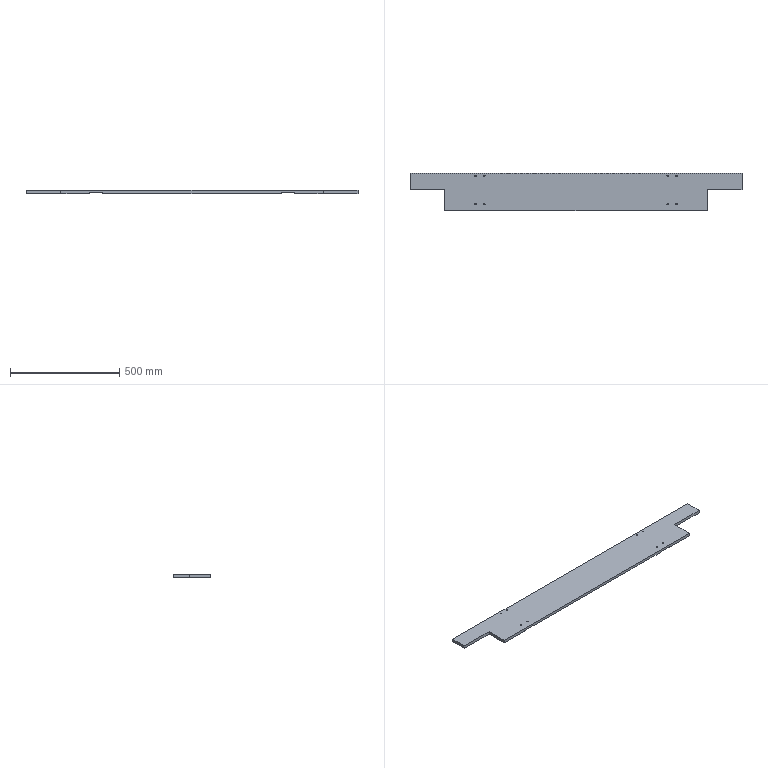Part | SolidWorks | features BaseBody 1 | 1 solid | 40 faces | box 1520 x 172 x 14 mm | volume 3159100 mm3 | cylinder 22 | plane 18 | commonest cylinder face diameters 6.8 x16 10 x6
STEP:
#1=CARTESIAN_POINT('',(-463.4,75.5,14.));
#2=VERTEX_POINT('',#1);
#3=CARTESIAN_POINT('',(-456.6,75.5,14.));
#4=VERTEX_POINT('',#3);
#5=CARTESIAN_POINT('',(-460.,75.5,14.));
#6=DIRECTION('',(0.,0.,1.));
#7=DIRECTION('',(1.,0.,0.));
#8=AXIS2_PLACEMENT_3D('',#5,#6,#7);
#9=CIRCLE('',#8,3.4);
#10=EDGE_CURVE('',#2,#4,#9,.T.);
#11=ORIENTED_EDGE('',*,*,#10,.T.);
#12=CARTESIAN_POINT('',(-456.6,75.5,3.));
#13=VERTEX_POINT('',#12);
#14=CARTESIAN_POINT('',(-456.6,75.5,3.));
#15=DIRECTION('',(0.,0.,-1.));
#16=VECTOR('',#15,1000.);
#17=LINE('',#14,#16);
#18=EDGE_CURVE('',#4,#13,#17,.T.);
#19=ORIENTED_EDGE('',*,*,#18,.T.);
#20=CARTESIAN_POINT('',(-463.4,75.5,3.));
#21=VERTEX_POINT('',#20);
#22=CARTESIAN_POINT('',(-460.,75.5,3.));
#23=DIRECTION('',(0.,0.,-1.));
#24=DIRECTION('',(-1.,0.,0.));
#25=AXIS2_PLACEMENT_3D('',#22,#23,#24);
#26=CIRCLE('',#25,3.4);
#27=EDGE_CURVE('',#13,#21,#26,.T.);
#28=ORIENTED_EDGE('',*,*,#27,.T.);
#29=CARTESIAN_POINT('',(-463.4,75.5,3.));
#30=DIRECTION('',(0.,0.,-1.));
#31=VECTOR('',#30,1000.);
#32=LINE('',#29,#31);
#33=EDGE_CURVE('',#2,#21,#32,.T.);
#34=ORIENTED_EDGE('',*,*,#33,.F.);
#35=EDGE_LOOP('',(#11,#19,#28,#34));
#36=FACE_OUTER_BOUND('',#35,.T.);
#37=CARTESIAN_POINT('',(-460.,75.5,3.));
#38=DIRECTION('',(0.,0.,-1.));
#39=DIRECTION('',(-1.,0.,0.));
#40=AXIS2_PLACEMENT_3D('',#37,#38,#39);
#41=CYLINDRICAL_SURFACE('',#40,3.4);
#42=ADVANCED_FACE('',(#36),#41,.F.);
#43=CARTESIAN_POINT('',(-423.4,75.5,14.));
#44=VERTEX_POINT('',#43);
#45=CARTESIAN_POINT('',(-416.6,75.5,14.));
#46=VERTEX_POINT('',#45);
#47=CARTESIAN_POINT('',(-420.,75.5,14.));
#48=DIRECTION('',(0.,0.,1.));
#49=DIRECTION('',(1.,0.,0.));
#50=AXIS2_PLACEMENT_3D('',#47,#48,#49);
#51=CIRCLE('',#50,3.4);
#52=EDGE_CURVE('',#44,#46,#51,.T.);
#53=ORIENTED_EDGE('',*,*,#52,.T.);
#54=CARTESIAN_POINT('',(-416.6,75.5,3.));
#55=VERTEX_POINT('',#54);
#56=CARTESIAN_POINT('',(-416.6,75.5,3.));
#57=DIRECTION('',(0.,0.,-1.));
#58=VECTOR('',#57,1000.);
#59=LINE('',#56,#58);
#60=EDGE_CURVE('',#46,#55,#59,.T.);
#61=ORIENTED_EDGE('',*,*,#60,.T.);
#62=CARTESIAN_POINT('',(-423.4,75.5,3.));
#63=VERTEX_POINT('',#62);
#64=CARTESIAN_POINT('',(-420.,75.5,3.));
#65=DIRECTION('',(0.,0.,-1.));
#66=DIRECTION('',(-1.,0.,0.));
#67=AXIS2_PLACEMENT_3D('',#64,#65,#66);
#68=CIRCLE('',#67,3.4);
#69=EDGE_CURVE('',#55,#63,#68,.T.);
#70=ORIENTED_EDGE('',*,*,#69,.T.);
#71=CARTESIAN_POINT('',(-423.4,75.5,3.));
#72=DIRECTION('',(0.,0.,-1.));
#73=VECTOR('',#72,1000.);
#74=LINE('',#71,#73);
#75=EDGE_CURVE('',#44,#63,#74,.T.);
#76=ORIENTED_EDGE('',*,*,#75,.F.);
#77=EDGE_LOOP('',(#53,#61,#70,#76));
#78=FACE_OUTER_BOUND('',#77,.T.);
#79=CARTESIAN_POINT('',(-420.,75.5,3.));
#80=DIRECTION('',(0.,0.,-1.));
#81=DIRECTION('',(-1.,0.,0.));
#82=AXIS2_PLACEMENT_3D('',#79,#80,#81);
#83=CYLINDRICAL_SURFACE('',#82,3.4);
#84=ADVANCED_FACE('',(#78),#83,.F.);
#85=CARTESIAN_POINT('',(-423.4,-54.5,14.));
#86=VERTEX_POINT('',#85);
#87=CARTESIAN_POINT('',(-416.6,-54.5,14.));
#88=VERTEX_POINT('',#87);
#89=CARTESIAN_POINT('',(-420.,-54.5,14.));
#90=DIRECTION('',(0.,0.,1.));
#91=DIRECTION('',(1.,0.,0.));
#92=AXIS2_PLACEMENT_3D('',#89,#90,#91);
#93=CIRCLE('',#92,3.4);
#94=EDGE_CURVE('',#86,#88,#93,.T.);
#95=ORIENTED_EDGE('',*,*,#94,.T.);
#96=CARTESIAN_POINT('',(-416.6,-54.5,3.));
#97=VERTEX_POINT('',#96);
#98=CARTESIAN_POINT('',(-416.6,-54.5,3.));
#99=DIRECTION('',(0.,0.,-1.));
#100=VECTOR('',#99,1000.);
#101=LINE('',#98,#100);
#102=EDGE_CURVE('',#88,#97,#101,.T.);
#103=ORIENTED_EDGE('',*,*,#102,.T.);
#104=CARTESIAN_POINT('',(-423.4,-54.5,3.));
#105=VERTEX_POINT('',#104);
#106=CARTESIAN_POINT('',(-420.,-54.5,3.));
#107=DIRECTION('',(0.,0.,-1.));
#108=DIRECTION('',(-1.,0.,0.));
#109=AXIS2_PLACEMENT_3D('',#106,#107,#108);
#110=CIRCLE('',#109,3.4);
#111=EDGE_CURVE('',#97,#105,#110,.T.);
#112=ORIENTED_EDGE('',*,*,#111,.T.);
#113=CARTESIAN_POINT('',(-423.4,-54.5,3.));
#114=DIRECTION('',(0.,0.,-1.));
#115=VECTOR('',#114,1000.);
#116=LINE('',#113,#115);
#117=EDGE_CURVE('',#86,#105,#116,.T.);
#118=ORIENTED_EDGE('',*,*,#117,.F.);
#119=EDGE_LOOP('',(#95,#103,#112,#118));
#120=FACE_OUTER_BOUND('',#119,.T.);
#121=CARTESIAN_POINT('',(-420.,-54.5,3.));
#122=DIRECTION('',(0.,0.,-1.));
#123=DIRECTION('',(-1.,0.,0.));
#124=AXIS2_PLACEMENT_3D('',#121,#122,#123);
#125=CYLINDRICAL_SURFACE('',#124,3.4);
#126=ADVANCED_FACE('',(#120),#125,.F.);
#127=CARTESIAN_POINT('',(-463.4,-54.5,14.));
#128=VERTEX_POINT('',#127);
#129=CARTESIAN_POINT('',(-456.6,-54.5,14.));
#130=VERTEX_POINT('',#129);
#131=CARTESIAN_POINT('',(-460.,-54.5,14.));
#132=DIRECTION('',(0.,0.,1.));
#133=DIRECTION('',(1.,0.,0.));
#134=AXIS2_PLACEMENT_3D('',#131,#132,#133);
#135=CIRCLE('',#134,3.4);
#136=EDGE_CURVE('',#128,#130,#135,.T.);
#137=ORIENTED_EDGE('',*,*,#136,.T.);
#138=CARTESIAN_POINT('',(-456.6,-54.5,3.));
#139=VERTEX_POINT('',#138);
#140=CARTESIAN_POINT('',(-456.6,-54.5,3.));
#141=DIRECTION('',(0.,0.,-1.));
#142=VECTOR('',#141,1000.);
#143=LINE('',#140,#142);
#144=EDGE_CURVE('',#130,#139,#143,.T.);
#145=ORIENTED_EDGE('',*,*,#144,.T.);
#146=CARTESIAN_POINT('',(-463.4,-54.5,3.));
#147=VERTEX_POINT('',#146);
#148=CARTESIAN_POINT('',(-460.,-54.5,3.));
#149=DIRECTION('',(0.,0.,-1.));
#150=DIRECTION('',(-1.,0.,0.));
#151=AXIS2_PLACEMENT_3D('',#148,#149,#150);
#152=CIRCLE('',#151,3.4);
#153=EDGE_CURVE('',#139,#147,#152,.T.);
#154=ORIENTED_EDGE('',*,*,#153,.T.);
#155=CARTESIAN_POINT('',(-463.4,-54.5,3.));
#156=DIRECTION('',(0.,0.,-1.));
#157=VECTOR('',#156,1000.);
#158=LINE('',#155,#157);
#159=EDGE_CURVE('',#128,#147,#158,.T.);
#160=ORIENTED_EDGE('',*,*,#159,.F.);
#161=EDGE_LOOP('',(#137,#145,#154,#160));
#162=FACE_OUTER_BOUND('',#161,.T.);
#163=CARTESIAN_POINT('',(-460.,-54.5,3.));
#164=DIRECTION('',(0.,0.,-1.));
#165=DIRECTION('',(-1.,0.,0.));
#166=AXIS2_PLACEMENT_3D('',#163,#164,#165);
#167=CYLINDRICAL_SURFACE('',#166,3.4);
#168=ADVANCED_FACE('',(#162),#167,.F.);
#169=CARTESIAN_POINT('',(416.6,75.5,14.));
#170=VERTEX_POINT('',#169);
#171=CARTESIAN_POINT('',(423.4,75.5,14.));
#172=VERTEX_POINT('',#171);
#173=CARTESIAN_POINT('',(420.,75.5,14.));
#174=DIRECTION('',(0.,0.,1.));
#175=DIRECTION('',(1.,0.,0.));
#176=AXIS2_PLACEMENT_3D('',#173,#174,#175);
#177=CIRCLE('',#176,3.4);
#178=EDGE_CURVE('',#170,#172,#177,.T.);
#179=ORIENTED_EDGE('',*,*,#178,.T.);
#180=CARTESIAN_POINT('',(423.4,75.5,3.));
#181=VERTEX_POINT('',#180);
#182=CARTESIAN_POINT('',(423.4,75.5,3.));
#183=DIRECTION('',(0.,0.,-1.));
#184=VECTOR('',#183,1000.);
#185=LINE('',#182,#184);
#186=EDGE_CURVE('',#172,#181,#185,.T.);
#187=ORIENTED_EDGE('',*,*,#186,.T.);
#188=CARTESIAN_POINT('',(416.6,75.5,3.));
#189=VERTEX_POINT('',#188);
#190=CARTESIAN_POINT('',(420.,75.5,3.));
#191=DIRECTION('',(0.,0.,-1.));
#192=DIRECTION('',(-1.,0.,0.));
#193=AXIS2_PLACEMENT_3D('',#190,#191,#192);
#194=CIRCLE('',#193,3.4);
#195=EDGE_CURVE('',#181,#189,#194,.T.);
#196=ORIENTED_EDGE('',*,*,#195,.T.);
#197=CARTESIAN_POINT('',(416.6,75.5,3.));
#198=DIRECTION('',(0.,0.,-1.));
#199=VECTOR('',#198,1000.);
#200=LINE('',#197,#199);
#201=EDGE_CURVE('',#170,#189,#200,.T.);
#202=ORIENTED_EDGE('',*,*,#201,.F.);
#203=EDGE_LOOP('',(#179,#187,#196,#202));
#204=FACE_OUTER_BOUND('',#203,.T.);
#205=CARTESIAN_POINT('',(420.,75.5,3.));
#206=DIRECTION('',(0.,0.,-1.));
#207=DIRECTION('',(-1.,0.,0.));
#208=AXIS2_PLACEMENT_3D('',#205,#206,#207);
#209=CYLINDRICAL_SURFACE('',#208,3.4);
#210=ADVANCED_FACE('',(#204),#209,.F.);
#211=CARTESIAN_POINT('',(456.6,75.5,14.));
#212=VERTEX_POINT('',#211);
#213=CARTESIAN_POINT('',(463.4,75.5,14.));
#214=VERTEX_POINT('',#213);
#215=CARTESIAN_POINT('',(460.,75.5,14.));
#216=DIRECTION('',(0.,0.,1.));
#217=DIRECTION('',(1.,0.,0.));
#218=AXIS2_PLACEMENT_3D('',#215,#216,#217);
#219=CIRCLE('',#218,3.4);
#220=EDGE_CURVE('',#212,#214,#219,.T.);
#221=ORIENTED_EDGE('',*,*,#220,.T.);
#222=CARTESIAN_POINT('',(463.4,75.5,3.));
#223=VERTEX_POINT('',#222);
#224=CARTESIAN_POINT('',(463.4,75.5,3.));
#225=DIRECTION('',(0.,0.,-1.));
#226=VECTOR('',#225,1000.);
#227=LINE('',#224,#226);
#228=EDGE_CURVE('',#214,#223,#227,.T.);
#229=ORIENTED_EDGE('',*,*,#228,.T.);
#230=CARTESIAN_POINT('',(456.6,75.5,3.));
#231=VERTEX_POINT('',#230);
#232=CARTESIAN_POINT('',(460.,75.5,3.));
#233=DIRECTION('',(0.,0.,-1.));
#234=DIRECTION('',(-1.,0.,0.));
#235=AXIS2_PLACEMENT_3D('',#232,#233,#234);
#236=CIRCLE('',#235,3.4);
#237=EDGE_CURVE('',#223,#231,#236,.T.);
#238=ORIENTED_EDGE('',*,*,#237,.T.);
#239=CARTESIAN_POINT('',(456.6,75.5,3.));
#240=DIRECTION('',(0.,0.,-1.));
#241=VECTOR('',#240,1000.);
#242=LINE('',#239,#241);
#243=EDGE_CURVE('',#212,#231,#242,.T.);
#244=ORIENTED_EDGE('',*,*,#243,.F.);
#245=EDGE_LOOP('',(#221,#229,#238,#244));
#246=FACE_OUTER_BOUND('',#245,.T.);
#247=CARTESIAN_POINT('',(460.,75.5,3.));
#248=DIRECTION('',(0.,0.,-1.));
#249=DIRECTION('',(-1.,0.,0.));
#250=AXIS2_PLACEMENT_3D('',#247,#248,#249);
#251=CYLINDRICAL_SURFACE('',#250,3.4);
#252=ADVANCED_FACE('',(#246),#251,.F.);
#253=CARTESIAN_POINT('',(456.6,-54.5,14.));
#254=VERTEX_POINT('',#253);
#255=CARTESIAN_POINT('',(463.4,-54.5,14.));
#256=VERTEX_POINT('',#255);
#257=CARTESIAN_POINT('',(460.,-54.5,14.));
#258=DIRECTION('',(0.,0.,1.));
#259=DIRECTION('',(1.,0.,0.));
#260=AXIS2_PLACEMENT_3D('',#257,#258,#259);
#261=CIRCLE('',#260,3.4);
#262=EDGE_CURVE('',#254,#256,#261,.T.);
#263=ORIENTED_EDGE('',*,*,#262,.T.);
#264=CARTESIAN_POINT('',(463.4,-54.5,3.));
#265=VERTEX_POINT('',#264);
#266=CARTESIAN_POINT('',(463.4,-54.5,3.));
#267=DIRECTION('',(0.,0.,-1.));
#268=VECTOR('',#267,1000.);
#269=LINE('',#266,#268);
#270=EDGE_CURVE('',#256,#265,#269,.T.);
#271=ORIENTED_EDGE('',*,*,#270,.T.);
#272=CARTESIAN_POINT('',(456.6,-54.5,3.));
#273=VERTEX_POINT('',#272);
#274=CARTESIAN_POINT('',(460.,-54.5,3.));
#275=DIRECTION('',(0.,0.,-1.));
#276=DIRECTION('',(-1.,0.,0.));
#277=AXIS2_PLACEMENT_3D('',#274,#275,#276);
#278=CIRCLE('',#277,3.4);
#279=EDGE_CURVE('',#265,#273,#278,.T.);
#280=ORIENTED_EDGE('',*,*,#279,.T.);
#281=CARTESIAN_POINT('',(456.6,-54.5,3.));
#282=DIRECTION('',(0.,0.,-1.));
#283=VECTOR('',#282,1000.);
#284=LINE('',#281,#283);
#285=EDGE_CURVE('',#254,#273,#284,.T.);
#286=ORIENTED_EDGE('',*,*,#285,.F.);
#287=EDGE_LOOP('',(#263,#271,#280,#286));
#288=FACE_OUTER_BOUND('',#287,.T.);
#289=CARTESIAN_POINT('',(460.,-54.5,3.));
#290=DIRECTION('',(0.,0.,-1.));
#291=DIRECTION('',(-1.,0.,0.));
#292=AXIS2_PLACEMENT_3D('',#289,#290,#291);
#293=CYLINDRICAL_SURFACE('',#292,3.4);
#294=ADVANCED_FACE('',(#288),#293,.F.);
#295=CARTESIAN_POINT('',(416.6,-54.5,14.));
#296=VERTEX_POINT('',#295);
#297=CARTESIAN_POINT('',(423.4,-54.5,14.));
#298=VERTEX_POINT('',#297);
#299=CARTESIAN_POINT('',(420.,-54.5,14.));
#300=DIRECTION('',(0.,0.,1.));
#301=DIRECTION('',(1.,0.,0.));
#302=AXIS2_PLACEMENT_3D('',#299,#300,#301);
#303=CIRCLE('',#302,3.4);
#304=EDGE_CURVE('',#296,#298,#303,.T.);
#305=ORIENTED_EDGE('',*,*,#304,.T.);
#306=CARTESIAN_POINT('',(423.4,-54.5,3.));
#307=VERTEX_POINT('',#306);
#308=CARTESIAN_POINT('',(423.4,-54.5,3.));
#309=DIRECTION('',(0.,0.,-1.));
#310=VECTOR('',#309,1000.);
#311=LINE('',#308,#310);
#312=EDGE_CURVE('',#298,#307,#311,.T.);
#313=ORIENTED_EDGE('',*,*,#312,.T.);
#314=CARTESIAN_POINT('',(416.6,-54.5,3.));
#315=VERTEX_POINT('',#314);
#316=CARTESIAN_POINT('',(420.,-54.5,3.));
#317=DIRECTION('',(0.,0.,-1.));
#318=DIRECTION('',(-1.,0.,0.));
#319=AXIS2_PLACEMENT_3D('',#316,#317,#318);
#320=CIRCLE('',#319,3.4);
#321=EDGE_CURVE('',#307,#315,#320,.T.);
#322=ORIENTED_EDGE('',*,*,#321,.T.);
#323=CARTESIAN_POINT('',(416.6,-54.5,3.));
#324=DIRECTION('',(0.,0.,-1.));
#325=VECTOR('',#324,1000.);
#326=LINE('',#323,#325);
#327=EDGE_CURVE('',#296,#315,#326,.T.);
#328=ORIENTED_EDGE('',*,*,#327,.F.);
#329=EDGE_LOOP('',(#305,#313,#322,#328));
#330=FACE_OUTER_BOUND('',#329,.T.);
#331=CARTESIAN_POINT('',(420.,-54.5,3.));
#332=DIRECTION('',(0.,0.,-1.));
#333=DIRECTION('',(-1.,0.,0.));
#334=AXIS2_PLACEMENT_3D('',#331,#332,#333);
#335=CYLINDRICAL_SURFACE('',#334,3.4);
#336=ADVANCED_FACE('',(#330),#335,.F.);
#337=CARTESIAN_POINT('',(-475.5,85.5,3.));
#338=VERTEX_POINT('',#337);
#339=CARTESIAN_POINT('',(-475.083,87.5,3.));
#340=VERTEX_POINT('',#339);
#341=CARTESIAN_POINT('',(-470.5,85.5,3.));
#342=DIRECTION('',(0.,0.,-1.));
#343=DIRECTION('',(1.,0.,0.));
#344=AXIS2_PLACEMENT_3D('',#341,#342,#343);
#345=CIRCLE('',#344,5.);
#346=EDGE_CURVE('',#338,#340,#345,.T.);
#347=ORIENTED_EDGE('',*,*,#346,.F.);
#348=CARTESIAN_POINT('',(-475.5,85.5,0.));
#349=VERTEX_POINT('',#348);
#350=CARTESIAN_POINT('',(-475.5,85.5,3.));
#351=DIRECTION('',(0.,0.,-1.));
#352=VECTOR('',#351,1000.);
#353=LINE('',#350,#352);
#354=EDGE_CURVE('',#338,#349,#353,.T.);
#355=ORIENTED_EDGE('',*,*,#354,.T.);
#356=CARTESIAN_POINT('',(-475.083,87.5,0.));
#357=VERTEX_POINT('',#356);
#358=CARTESIAN_POINT('',(-470.5,85.5,0.));
#359=DIRECTION('',(0.,0.,1.));
#360=DIRECTION('',(1.,0.,0.));
#361=AXIS2_PLACEMENT_3D('',#358,#359,#360);
#362=CIRCLE('',#361,5.);
#363=EDGE_CURVE('',#357,#349,#362,.T.);
#364=ORIENTED_EDGE('',*,*,#363,.F.);
#365=CARTESIAN_POINT('',(-475.083,87.5,3.));
#366=DIRECTION('',(0.,0.,-1.));
#367=VECTOR('',#366,1000.);
#368=LINE('',#365,#367);
#369=EDGE_CURVE('',#340,#357,#368,.T.);
#370=ORIENTED_EDGE('',*,*,#369,.F.);
#371=EDGE_LOOP('',(#347,#355,#364,#370));
#372=FACE_OUTER_BOUND('',#371,.T.);
#373=CARTESIAN_POINT('',(-470.5,85.5,3.));
#374=DIRECTION('',(0.,0.,-1.));
#375=DIRECTION('',(-1.,0.,0.));
#376=AXIS2_PLACEMENT_3D('',#373,#374,#375);
#377=CYLINDRICAL_SURFACE('',#376,5.);
#378=ADVANCED_FACE('',(#372),#377,.F.);
#379=CARTESIAN_POINT('',(404.5,85.5,3.));
#380=VERTEX_POINT('',#379);
#381=CARTESIAN_POINT('',(404.917,87.5,3.));
#382=VERTEX_POINT('',#381);
#383=CARTESIAN_POINT('',(409.5,85.5,3.));
#384=DIRECTION('',(0.,0.,-1.));
#385=DIRECTION('',(-1.,0.,0.));
#386=AXIS2_PLACEMENT_3D('',#383,#384,#385);
#387=CIRCLE('',#386,5.);
#388=EDGE_CURVE('',#380,#382,#387,.T.);
#389=ORIENTED_EDGE('',*,*,#388,.F.);
#390=CARTESIAN_POINT('',(404.5,85.5,0.));
#391=VERTEX_POINT('',#390);
#392=CARTESIAN_POINT('',(404.5,85.5,3.));
#393=DIRECTION('',(0.,0.,-1.));
#394=VECTOR('',#393,1000.);
#395=LINE('',#392,#394);
#396=EDGE_CURVE('',#380,#391,#395,.T.);
#397=ORIENTED_EDGE('',*,*,#396,.T.);
#398=CARTESIAN_POINT('',(404.917,87.5,0.));
#399=VERTEX_POINT('',#398);
#400=CARTESIAN_POINT('',(409.5,85.5,0.));
#401=DIRECTION('',(0.,0.,1.));
#402=DIRECTION('',(1.,0.,0.));
#403=AXIS2_PLACEMENT_3D('',#400,#401,#402);
#404=CIRCLE('',#403,5.);
#405=EDGE_CURVE('',#399,#391,#404,.T.);
#406=ORIENTED_EDGE('',*,*,#405,.F.);
#407=CARTESIAN_POINT('',(404.917,87.5,3.));
#408=DIRECTION('',(0.,0.,-1.));
#409=VECTOR('',#408,1000.);
#410=LINE('',#407,#409);
#411=EDGE_CURVE('',#382,#399,#410,.T.);
#412=ORIENTED_EDGE('',*,*,#411,.F.);
#413=EDGE_LOOP('',(#389,#397,#406,#412));
#414=FACE_OUTER_BOUND('',#413,.T.);
#415=CARTESIAN_POINT('',(409.5,85.5,3.));
#416=DIRECTION('',(0.,0.,-1.));
#417=DIRECTION('',(-1.,0.,0.));
#418=AXIS2_PLACEMENT_3D('',#415,#416,#417);
#419=CYLINDRICAL_SURFACE('',#418,5.);
#420=ADVANCED_FACE('',(#414),#419,.F.);
#421=CARTESIAN_POINT('',(-409.5,80.5,0.));
#422=VERTEX_POINT('',#421);
#423=CARTESIAN_POINT('',(-409.5,-84.5,0.));
#424=VERTEX_POINT('',#423);
#425=CARTESIAN_POINT('',(-409.5,0.,0.));
#426=DIRECTION('',(0.,-1.,0.));
#427=VECTOR('',#426,1000.);
#428=LINE('',#425,#427);
#429=EDGE_CURVE('',#422,#424,#428,.T.);
#430=ORIENTED_EDGE('',*,*,#429,.F.);
#431=CARTESIAN_POINT('',(-404.917,87.5,0.));
#432=VERTEX_POINT('',#431);
#433=CARTESIAN_POINT('',(-409.5,85.5,0.));
#434=DIRECTION('',(0.,0.,1.));
#435=DIRECTION('',(1.,0.,0.));
#436=AXIS2_PLACEMENT_3D('',#433,#434,#435);
#437=CIRCLE('',#436,5.);
#438=EDGE_CURVE('',#422,#432,#437,.T.);
#439=ORIENTED_EDGE('',*,*,#438,.T.);
#440=CARTESIAN_POINT('',(-760.,87.5,0.));
#441=DIRECTION('',(-1.,0.,0.));
#442=VECTOR('',#441,1000.);
#443=LINE('',#440,#442);
#444=EDGE_CURVE('',#399,#432,#443,.T.);
#445=ORIENTED_EDGE('',*,*,#444,.F.);
#446=ORIENTED_EDGE('',*,*,#405,.T.);
#447=CARTESIAN_POINT('',(409.5,80.5,0.));
#448=VERTEX_POINT('',#447);
#449=CARTESIAN_POINT('',(409.5,85.5,0.));
#450=DIRECTION('',(0.,0.,1.));
#451=DIRECTION('',(1.,0.,0.));
#452=AXIS2_PLACEMENT_3D('',#449,#450,#451);
#453=CIRCLE('',#452,5.);
#454=EDGE_CURVE('',#391,#448,#453,.T.);
#455=ORIENTED_EDGE('',*,*,#454,.T.);
#456=CARTESIAN_POINT('',(409.5,-84.5,0.));
#457=VERTEX_POINT('',#456);
#458=CARTESIAN_POINT('',(409.5,0.,0.));
#459=DIRECTION('',(0.,1.,0.));
#460=VECTOR('',#459,1000.);
#461=LINE('',#458,#460);
#462=EDGE_CURVE('',#457,#448,#461,.T.);
#463=ORIENTED_EDGE('',*,*,#462,.F.);
#464=CARTESIAN_POINT('',(-600.,-84.5,0.));
#465=DIRECTION('',(1.,0.,0.));
#466=VECTOR('',#465,1000.);
#467=LINE('',#464,#466);
#468=EDGE_CURVE('',#424,#457,#467,.T.);
#469=ORIENTED_EDGE('',*,*,#468,.F.);
#470=EDGE_LOOP('',(#430,#439,#445,#446,#455,#463,#469));
#471=FACE_OUTER_BOUND('',#470,.T.);
#472=CARTESIAN_POINT('',(0.,0.,0.));
#473=DIRECTION('',(0.,0.,1.));
#474=DIRECTION('',(1.,0.,0.));
#475=AXIS2_PLACEMENT_3D('',#472,#473,#474);
#476=PLANE('',#475);
#477=ADVANCED_FACE('',(#471),#476,.F.);
#478=CARTESIAN_POINT('',(470.5,80.5,0.));
#479=VERTEX_POINT('',#478);
#480=CARTESIAN_POINT('',(470.5,-84.5,0.));
#481=VERTEX_POINT('',#480);
#482=CARTESIAN_POINT('',(470.5,0.,0.));
#483=DIRECTION('',(0.,-1.,0.));
#484=VECTOR('',#483,1000.);
#485=LINE('',#482,#484);
#486=EDGE_CURVE('',#479,#481,#485,.T.);
#487=ORIENTED_EDGE('',*,*,#486,.F.);
#488=CARTESIAN_POINT('',(475.083,87.5,0.));
#489=VERTEX_POINT('',#488);
#490=CARTESIAN_POINT('',(470.5,85.5,0.));
#491=DIRECTION('',(0.,0.,1.));
#492=DIRECTION('',(1.,0.,0.));
#493=AXIS2_PLACEMENT_3D('',#490,#491,#492);
#494=CIRCLE('',#493,5.);
#495=EDGE_CURVE('',#479,#489,#494,.T.);
#496=ORIENTED_EDGE('',*,*,#495,.T.);
#497=CARTESIAN_POINT('',(760.,87.5,0.));
#498=VERTEX_POINT('',#497);
#499=CARTESIAN_POINT('',(-760.,87.5,0.));
#500=DIRECTION('',(-1.,0.,0.));
#501=VECTOR('',#500,1000.);
#502=LINE('',#499,#501);
#503=EDGE_CURVE('',#498,#489,#502,.T.);
#504=ORIENTED_EDGE('',*,*,#503,.F.);
#505=CARTESIAN_POINT('',(760.,12.5,0.));
#506=VERTEX_POINT('',#505);
#507=CARTESIAN_POINT('',(760.,87.5,0.));
#508=DIRECTION('',(0.,1.,0.));
#509=VECTOR('',#508,1000.);
#510=LINE('',#507,#509);
#511=EDGE_CURVE('',#506,#498,#510,.T.);
#512=ORIENTED_EDGE('',*,*,#511,.F.);
#513=CARTESIAN_POINT('',(600.,12.5,0.));
#514=VERTEX_POINT('',#513);
#515=CARTESIAN_POINT('',(760.,12.5,0.));
#516=DIRECTION('',(-1.,0.,0.));
#517=VECTOR('',#516,1000.);
#518=LINE('',#515,#517);
#519=EDGE_CURVE('',#506,#514,#518,.T.);
#520=ORIENTED_EDGE('',*,*,#519,.T.);
#521=CARTESIAN_POINT('',(600.,-84.5,0.));
#522=VERTEX_POINT('',#521);
#523=CARTESIAN_POINT('',(600.,12.5,0.));
#524=DIRECTION('',(0.,-1.,0.));
#525=VECTOR('',#524,1000.);
#526=LINE('',#523,#525);
#527=EDGE_CURVE('',#514,#522,#526,.T.);
#528=ORIENTED_EDGE('',*,*,#527,.T.);
#529=CARTESIAN_POINT('',(-600.,-84.5,0.));
#530=DIRECTION('',(1.,0.,0.));
#531=VECTOR('',#530,1000.);
#532=LINE('',#529,#531);
#533=EDGE_CURVE('',#481,#522,#532,.T.);
#534=ORIENTED_EDGE('',*,*,#533,.F.);
#535=EDGE_LOOP('',(#487,#496,#504,#512,#520,#528,#534));
#536=FACE_OUTER_BOUND('',#535,.T.);
#537=CARTESIAN_POINT('',(0.,0.,0.));
#538=DIRECTION('',(0.,0.,1.));
#539=DIRECTION('',(1.,0.,0.));
#540=AXIS2_PLACEMENT_3D('',#537,#538,#539);
#541=PLANE('',#540);
#542=ADVANCED_FACE('',(#536),#541,.F.);
#543=ORIENTED_EDGE('',*,*,#444,.T.);
#544=CARTESIAN_POINT('',(-404.917,87.5,3.));
#545=VERTEX_POINT('',#544);
#546=CARTESIAN_POINT('',(-404.917,87.5,3.));
#547=DIRECTION('',(0.,0.,1.));
#548=VECTOR('',#547,1000.);
#549=LINE('',#546,#548);
#550=EDGE_CURVE('',#432,#545,#549,.T.);
#551=ORIENTED_EDGE('',*,*,#550,.T.);
#552=CARTESIAN_POINT('',(-760.,87.5,3.));
#553=DIRECTION('',(-1.,0.,0.));
#554=VECTOR('',#553,1000.);
#555=LINE('',#552,#554);
#556=EDGE_CURVE('',#545,#340,#555,.T.);
#557=ORIENTED_EDGE('',*,*,#556,.T.);
#558=ORIENTED_EDGE('',*,*,#369,.T.);
#559=CARTESIAN_POINT('',(-760.,87.5,0.));
#560=VERTEX_POINT('',#559);
#561=CARTESIAN_POINT('',(-760.,87.5,0.));
#562=DIRECTION('',(-1.,0.,0.));
#563=VECTOR('',#562,1000.);
#564=LINE('',#561,#563);
#565=EDGE_CURVE('',#357,#560,#564,.T.);
#566=ORIENTED_EDGE('',*,*,#565,.T.);
#567=CARTESIAN_POINT('',(-760.,87.5,14.));
#568=VERTEX_POINT('',#567);
#569=CARTESIAN_POINT('',(-760.,87.5,14.));
#570=DIRECTION('',(0.,0.,-1.));
#571=VECTOR('',#570,1000.);
#572=LINE('',#569,#571);
#573=EDGE_CURVE('',#568,#560,#572,.T.);
#574=ORIENTED_EDGE('',*,*,#573,.F.);
#575=CARTESIAN_POINT('',(760.,87.5,14.));
#576=VERTEX_POINT('',#575);
#577=CARTESIAN_POINT('',(-760.,87.5,14.));
#578=DIRECTION('',(-1.,0.,0.));
#579=VECTOR('',#578,1000.);
#580=LINE('',#577,#579);
#581=EDGE_CURVE('',#576,#568,#580,.T.);
#582=ORIENTED_EDGE('',*,*,#581,.F.);
#583=CARTESIAN_POINT('',(760.,87.5,14.));
#584=DIRECTION('',(0.,0.,-1.));
#585=VECTOR('',#584,1000.);
#586=LINE('',#583,#585);
#587=EDGE_CURVE('',#576,#498,#586,.T.);
#588=ORIENTED_EDGE('',*,*,#587,.T.);
#589=ORIENTED_EDGE('',*,*,#503,.T.);
#590=CARTESIAN_POINT('',(475.083,87.5,3.));
#591=VERTEX_POINT('',#590);
#592=CARTESIAN_POINT('',(475.083,87.5,3.));
#593=DIRECTION('',(0.,0.,1.));
#594=VECTOR('',#593,1000.);
#595=LINE('',#592,#594);
#596=EDGE_CURVE('',#489,#591,#595,.T.);
#597=ORIENTED_EDGE('',*,*,#596,.T.);
#598=CARTESIAN_POINT('',(-760.,87.5,3.));
#599=DIRECTION('',(-1.,0.,0.));
#600=VECTOR('',#599,1000.);
#601=LINE('',#598,#600);
#602=EDGE_CURVE('',#591,#382,#601,.T.);
#603=ORIENTED_EDGE('',*,*,#602,.T.);
#604=ORIENTED_EDGE('',*,*,#411,.T.);
#605=EDGE_LOOP('',(#543,#551,#557,#558,#566,#574,#582,#588,#589,#597,#603,#604));
#606=FACE_OUTER_BOUND('',#605,.T.);
#607=CARTESIAN_POINT('',(-760.,87.5,14.));
#608=DIRECTION('',(0.,-1.,0.));
#609=DIRECTION('',(0.,0.,-1.));
#610=AXIS2_PLACEMENT_3D('',#607,#608,#609);
#611=PLANE('',#610);
#612=ADVANCED_FACE('',(#606),#611,.F.);
#613=ORIENTED_EDGE('',*,*,#468,.T.);
#614=CARTESIAN_POINT('',(409.5,-84.5,3.));
#615=VERTEX_POINT('',#614);
#616=CARTESIAN_POINT('',(409.5,-84.5,3.));
#617=DIRECTION('',(0.,0.,-1.));
#618=VECTOR('',#617,1000.);
#619=LINE('',#616,#618);
#620=EDGE_CURVE('',#615,#457,#619,.T.);
#621=ORIENTED_EDGE('',*,*,#620,.F.);
#622=CARTESIAN_POINT('',(470.5,-84.5,3.));
#623=VERTEX_POINT('',#622);
#624=CARTESIAN_POINT('',(470.5,-84.5,3.));
#625=DIRECTION('',(1.,0.,0.));
#626=VECTOR('',#625,1000.);
#627=LINE('',#624,#626);
#628=EDGE_CURVE('',#615,#623,#627,.T.);
#629=ORIENTED_EDGE('',*,*,#628,.T.);
#630=CARTESIAN_POINT('',(470.5,-84.5,3.));
#631=DIRECTION('',(0.,0.,-1.));
#632=VECTOR('',#631,1000.);
#633=LINE('',#630,#632);
#634=EDGE_CURVE('',#623,#481,#633,.T.);
#635=ORIENTED_EDGE('',*,*,#634,.T.);
#636=ORIENTED_EDGE('',*,*,#533,.T.);
#637=CARTESIAN_POINT('',(600.,-84.5,14.));
#638=VERTEX_POINT('',#637);
#639=CARTESIAN_POINT('',(600.,-84.5,140.));
#640=DIRECTION('',(0.,0.,1.));
#641=VECTOR('',#640,1000.);
#642=LINE('',#639,#641);
#643=EDGE_CURVE('',#522,#638,#642,.T.);
#644=ORIENTED_EDGE('',*,*,#643,.T.);
#645=CARTESIAN_POINT('',(-600.,-84.5,14.));
#646=VERTEX_POINT('',#645);
#647=CARTESIAN_POINT('',(0.,-84.5,14.));
#648=DIRECTION('',(1.,0.,0.));
#649=VECTOR('',#648,1000.);
#650=LINE('',#647,#649);
#651=EDGE_CURVE('',#646,#638,#650,.T.);
#652=ORIENTED_EDGE('',*,*,#651,.F.);
#653=CARTESIAN_POINT('',(-600.,-84.5,0.));
#654=VERTEX_POINT('',#653);
#655=CARTESIAN_POINT('',(-600.,-84.5,0.));
#656=DIRECTION('',(0.,0.,-1.));
#657=VECTOR('',#656,1000.);
#658=LINE('',#655,#657);
#659=EDGE_CURVE('',#646,#654,#658,.T.);
#660=ORIENTED_EDGE('',*,*,#659,.T.);
#661=CARTESIAN_POINT('',(-470.5,-84.5,0.));
#662=VERTEX_POINT('',#661);
#663=CARTESIAN_POINT('',(-600.,-84.5,0.));
#664=DIRECTION('',(1.,0.,0.));
#665=VECTOR('',#664,1000.);
#666=LINE('',#663,#665);
#667=EDGE_CURVE('',#654,#662,#666,.T.);
#668=ORIENTED_EDGE('',*,*,#667,.T.);
#669=CARTESIAN_POINT('',(-470.5,-84.5,3.));
#670=VERTEX_POINT('',#669);
#671=CARTESIAN_POINT('',(-470.5,-84.5,3.));
#672=DIRECTION('',(0.,0.,-1.));
#673=VECTOR('',#672,1000.);
#674=LINE('',#671,#673);
#675=EDGE_CURVE('',#670,#662,#674,.T.);
#676=ORIENTED_EDGE('',*,*,#675,.F.);
#677=CARTESIAN_POINT('',(-409.5,-84.5,3.));
#678=VERTEX_POINT('',#677);
#679=CARTESIAN_POINT('',(-470.5,-84.5,3.));
#680=DIRECTION('',(1.,0.,0.));
#681=VECTOR('',#680,1000.);
#682=LINE('',#679,#681);
#683=EDGE_CURVE('',#670,#678,#682,.T.);
#684=ORIENTED_EDGE('',*,*,#683,.T.);
#685=CARTESIAN_POINT('',(-409.5,-84.5,3.));
#686=DIRECTION('',(0.,0.,-1.));
#687=VECTOR('',#686,1000.);
#688=LINE('',#685,#687);
#689=EDGE_CURVE('',#678,#424,#688,.T.);
#690=ORIENTED_EDGE('',*,*,#689,.T.);
#691=EDGE_LOOP('',(#613,#621,#629,#635,#636,#644,#652,#660,#668,#676,#684,#690));
#692=FACE_OUTER_BOUND('',#691,.T.);
#693=CARTESIAN_POINT('',(0.,-84.5,70.));
#694=DIRECTION('',(0.,-1.,0.));
#695=DIRECTION('',(0.,0.,-1.));
#696=AXIS2_PLACEMENT_3D('',#693,#694,#695);
#697=PLANE('',#696);
#698=ADVANCED_FACE('',(#692),#697,.T.);
#699=ORIENTED_EDGE('',*,*,#565,.F.);
#700=ORIENTED_EDGE('',*,*,#363,.T.);
#701=CARTESIAN_POINT('',(-470.5,80.5,0.));
#702=VERTEX_POINT('',#701);
#703=CARTESIAN_POINT('',(-470.5,85.5,0.));
#704=DIRECTION('',(0.,0.,1.));
#705=DIRECTION('',(1.,0.,0.));
#706=AXIS2_PLACEMENT_3D('',#703,#704,#705);
#707=CIRCLE('',#706,5.);
#708=EDGE_CURVE('',#349,#702,#707,.T.);
#709=ORIENTED_EDGE('',*,*,#708,.T.);
#710=CARTESIAN_POINT('',(-470.5,0.,0.));
#711=DIRECTION('',(0.,1.,0.));
#712=VECTOR('',#711,1000.);
#713=LINE('',#710,#712);
#714=EDGE_CURVE('',#662,#702,#713,.T.);
#715=ORIENTED_EDGE('',*,*,#714,.F.);
#716=ORIENTED_EDGE('',*,*,#667,.F.);
#717=CARTESIAN_POINT('',(-600.,12.5,0.));
#718=VERTEX_POINT('',#717);
#719=CARTESIAN_POINT('',(-600.,12.5,0.));
#720=DIRECTION('',(0.,1.,0.));
#721=VECTOR('',#720,1000.);
#722=LINE('',#719,#721);
#723=EDGE_CURVE('',#654,#718,#722,.T.);
#724=ORIENTED_EDGE('',*,*,#723,.T.);
#725=CARTESIAN_POINT('',(-760.,12.5,0.));
#726=VERTEX_POINT('',#725);
#727=CARTESIAN_POINT('',(-760.,12.5,0.));
#728=DIRECTION('',(-1.,0.,0.));
#729=VECTOR('',#728,1000.);
#730=LINE('',#727,#729);
#731=EDGE_CURVE('',#718,#726,#730,.T.);
#732=ORIENTED_EDGE('',*,*,#731,.T.);
#733=CARTESIAN_POINT('',(-760.,87.5,0.));
#734=DIRECTION('',(0.,-1.,0.));
#735=VECTOR('',#734,1000.);
#736=LINE('',#733,#735);
#737=EDGE_CURVE('',#560,#726,#736,.T.);
#738=ORIENTED_EDGE('',*,*,#737,.F.);
#739=EDGE_LOOP('',(#699,#700,#709,#715,#716,#724,#732,#738));
#740=FACE_OUTER_BOUND('',#739,.T.);
#741=CARTESIAN_POINT('',(0.,0.,0.));
#742=DIRECTION('',(0.,0.,1.));
#743=DIRECTION('',(1.,0.,0.));
#744=AXIS2_PLACEMENT_3D('',#741,#742,#743);
#745=PLANE('',#744);
#746=ADVANCED_FACE('',(#740),#745,.F.);
#747=ORIENTED_EDGE('',*,*,#10,.F.);
#748=CARTESIAN_POINT('',(-460.,75.5,14.));
#749=DIRECTION('',(0.,0.,1.));
#750=DIRECTION('',(1.,0.,0.));
#751=AXIS2_PLACEMENT_3D('',#748,#749,#750);
#752=CIRCLE('',#751,3.4);
#753=EDGE_CURVE('',#4,#2,#752,.T.);
#754=ORIENTED_EDGE('',*,*,#753,.F.);
#755=EDGE_LOOP('',(#747,#754));
#756=FACE_BOUND('',#755,.T.);
#757=ORIENTED_EDGE('',*,*,#52,.F.);
#758=CARTESIAN_POINT('',(-420.,75.5,14.));
#759=DIRECTION('',(0.,0.,1.));
#760=DIRECTION('',(1.,0.,0.));
#761=AXIS2_PLACEMENT_3D('',#758,#759,#760);
#762=CIRCLE('',#761,3.4);
#763=EDGE_CURVE('',#46,#44,#762,.T.);
#764=ORIENTED_EDGE('',*,*,#763,.F.);
#765=EDGE_LOOP('',(#757,#764));
#766=FACE_BOUND('',#765,.T.);
#767=ORIENTED_EDGE('',*,*,#94,.F.);
#768=CARTESIAN_POINT('',(-420.,-54.5,14.));
#769=DIRECTION('',(0.,0.,1.));
#770=DIRECTION('',(1.,0.,0.));
#771=AXIS2_PLACEMENT_3D('',#768,#769,#770);
#772=CIRCLE('',#771,3.4);
#773=EDGE_CURVE('',#88,#86,#772,.T.);
#774=ORIENTED_EDGE('',*,*,#773,.F.);
#775=EDGE_LOOP('',(#767,#774));
#776=FACE_BOUND('',#775,.T.);
#777=ORIENTED_EDGE('',*,*,#136,.F.);
#778=CARTESIAN_POINT('',(-460.,-54.5,14.));
#779=DIRECTION('',(0.,0.,1.));
#780=DIRECTION('',(1.,0.,0.));
#781=AXIS2_PLACEMENT_3D('',#778,#779,#780);
#782=CIRCLE('',#781,3.4);
#783=EDGE_CURVE('',#130,#128,#782,.T.);
#784=ORIENTED_EDGE('',*,*,#783,.F.);
#785=EDGE_LOOP('',(#777,#784));
#786=FACE_BOUND('',#785,.T.);
#787=ORIENTED_EDGE('',*,*,#178,.F.);
#788=CARTESIAN_POINT('',(420.,75.5,14.));
#789=DIRECTION('',(0.,0.,1.));
#790=DIRECTION('',(1.,0.,0.));
#791=AXIS2_PLACEMENT_3D('',#788,#789,#790);
#792=CIRCLE('',#791,3.4);
#793=EDGE_CURVE('',#172,#170,#792,.T.);
#794=ORIENTED_EDGE('',*,*,#793,.F.);
#795=EDGE_LOOP('',(#787,#794));
#796=FACE_BOUND('',#795,.T.);
#797=ORIENTED_EDGE('',*,*,#220,.F.);
#798=CARTESIAN_POINT('',(460.,75.5,14.));
#799=DIRECTION('',(0.,0.,1.));
#800=DIRECTION('',(1.,0.,0.));
#801=AXIS2_PLACEMENT_3D('',#798,#799,#800);
#802=CIRCLE('',#801,3.4);
#803=EDGE_CURVE('',#214,#212,#802,.T.);
#804=ORIENTED_EDGE('',*,*,#803,.F.);
#805=EDGE_LOOP('',(#797,#804));
#806=FACE_BOUND('',#805,.T.);
#807=ORIENTED_EDGE('',*,*,#262,.F.);
#808=CARTESIAN_POINT('',(460.,-54.5,14.));
#809=DIRECTION('',(0.,0.,1.));
#810=DIRECTION('',(1.,0.,0.));
#811=AXIS2_PLACEMENT_3D('',#808,#809,#810);
#812=CIRCLE('',#811,3.4);
#813=EDGE_CURVE('',#256,#254,#812,.T.);
#814=ORIENTED_EDGE('',*,*,#813,.F.);
#815=EDGE_LOOP('',(#807,#814));
#816=FACE_BOUND('',#815,.T.);
#817=ORIENTED_EDGE('',*,*,#304,.F.);
#818=CARTESIAN_POINT('',(420.,-54.5,14.));
#819=DIRECTION('',(0.,0.,1.));
#820=DIRECTION('',(1.,0.,0.));
#821=AXIS2_PLACEMENT_3D('',#818,#819,#820);
#822=CIRCLE('',#821,3.4);
#823=EDGE_CURVE('',#298,#296,#822,.T.);
#824=ORIENTED_EDGE('',*,*,#823,.F.);
#825=EDGE_LOOP('',(#817,#824));
#826=FACE_BOUND('',#825,.T.);
#827=CARTESIAN_POINT('',(-600.,12.5,14.));
#828=VERTEX_POINT('',#827);
#829=CARTESIAN_POINT('',(-600.,12.5,14.));
#830=DIRECTION('',(0.,1.,0.));
#831=VECTOR('',#830,1000.);
#832=LINE('',#829,#831);
#833=EDGE_CURVE('',#646,#828,#832,.T.);
#834=ORIENTED_EDGE('',*,*,#833,.F.);
#835=ORIENTED_EDGE('',*,*,#651,.T.);
#836=CARTESIAN_POINT('',(600.,12.5,14.));
#837=VERTEX_POINT('',#836);
#838=CARTESIAN_POINT('',(600.,12.5,14.));
#839=DIRECTION('',(0.,-1.,0.));
#840=VECTOR('',#839,1000.);
#841=LINE('',#838,#840);
#842=EDGE_CURVE('',#837,#638,#841,.T.);
#843=ORIENTED_EDGE('',*,*,#842,.F.);
#844=CARTESIAN_POINT('',(760.,12.5,14.));
#845=VERTEX_POINT('',#844);
#846=CARTESIAN_POINT('',(760.,12.5,14.));
#847=DIRECTION('',(-1.,0.,0.));
#848=VECTOR('',#847,1000.);
#849=LINE('',#846,#848);
#850=EDGE_CURVE('',#845,#837,#849,.T.);
#851=ORIENTED_EDGE('',*,*,#850,.F.);
#852=CARTESIAN_POINT('',(760.,87.5,14.));
#853=DIRECTION('',(0.,1.,0.));
#854=VECTOR('',#853,1000.);
#855=LINE('',#852,#854);
#856=EDGE_CURVE('',#845,#576,#855,.T.);
#857=ORIENTED_EDGE('',*,*,#856,.T.);
#858=ORIENTED_EDGE('',*,*,#581,.T.);
#859=CARTESIAN_POINT('',(-760.,12.5,14.));
#860=VERTEX_POINT('',#859);
#861=CARTESIAN_POINT('',(-760.,87.5,14.));
#862=DIRECTION('',(0.,-1.,0.));
#863=VECTOR('',#862,1000.);
#864=LINE('',#861,#863);
#865=EDGE_CURVE('',#568,#860,#864,.T.);
#866=ORIENTED_EDGE('',*,*,#865,.T.);
#867=CARTESIAN_POINT('',(-760.,12.5,14.));
#868=DIRECTION('',(-1.,0.,0.));
#869=VECTOR('',#868,1000.);
#870=LINE('',#867,#869);
#871=EDGE_CURVE('',#828,#860,#870,.T.);
#872=ORIENTED_EDGE('',*,*,#871,.F.);
#873=EDGE_LOOP('',(#834,#835,#843,#851,#857,#858,#866,#872));
#874=FACE_OUTER_BOUND('',#873,.T.);
#875=CARTESIAN_POINT('',(0.,0.,14.));
#876=DIRECTION('',(0.,0.,1.));
#877=DIRECTION('',(1.,0.,0.));
#878=AXIS2_PLACEMENT_3D('',#875,#876,#877);
#879=PLANE('',#878);
#880=ADVANCED_FACE('',(#756,#766,#776,#786,#796,#806,#816,#826,#874),#879,.T.);
#881=ORIENTED_EDGE('',*,*,#643,.F.);
#882=ORIENTED_EDGE('',*,*,#527,.F.);
#883=CARTESIAN_POINT('',(600.,12.5,0.));
#884=DIRECTION('',(0.,0.,1.));
#885=VECTOR('',#884,1000.);
#886=LINE('',#883,#885);
#887=EDGE_CURVE('',#514,#837,#886,.T.);
#888=ORIENTED_EDGE('',*,*,#887,.T.);
#889=ORIENTED_EDGE('',*,*,#842,.T.);
#890=EDGE_LOOP('',(#881,#882,#888,#889));
#891=FACE_OUTER_BOUND('',#890,.T.);
#892=CARTESIAN_POINT('',(600.,12.5,0.));
#893=DIRECTION('',(-1.,0.,0.));
#894=DIRECTION('',(0.,0.,1.));
#895=AXIS2_PLACEMENT_3D('',#892,#893,#894);
#896=PLANE('',#895);
#897=ADVANCED_FACE('',(#891),#896,.F.);
#898=ORIENTED_EDGE('',*,*,#659,.F.);
#899=ORIENTED_EDGE('',*,*,#833,.T.);
#900=CARTESIAN_POINT('',(-600.,12.5,0.));
#901=DIRECTION('',(0.,0.,1.));
#902=VECTOR('',#901,1000.);
#903=LINE('',#900,#902);
#904=EDGE_CURVE('',#718,#828,#903,.T.);
#905=ORIENTED_EDGE('',*,*,#904,.F.);
#906=ORIENTED_EDGE('',*,*,#723,.F.);
#907=EDGE_LOOP('',(#898,#899,#905,#906));
#908=FACE_OUTER_BOUND('',#907,.T.);
#909=CARTESIAN_POINT('',(-600.,12.5,0.));
#910=DIRECTION('',(1.,0.,0.));
#911=DIRECTION('',(0.,0.,-1.));
#912=AXIS2_PLACEMENT_3D('',#909,#910,#911);
#913=PLANE('',#912);
#914=ADVANCED_FACE('',(#908),#913,.F.);
#915=ORIENTED_EDGE('',*,*,#856,.F.);
#916=CARTESIAN_POINT('',(760.,12.5,0.));
#917=DIRECTION('',(0.,0.,1.));
#918=VECTOR('',#917,1000.);
#919=LINE('',#916,#918);
#920=EDGE_CURVE('',#506,#845,#919,.T.);
#921=ORIENTED_EDGE('',*,*,#920,.F.);
#922=ORIENTED_EDGE('',*,*,#511,.T.);
#923=ORIENTED_EDGE('',*,*,#587,.F.);
#924=EDGE_LOOP('',(#915,#921,#922,#923));
#925=FACE_OUTER_BOUND('',#924,.T.);
#926=CARTESIAN_POINT('',(760.,87.5,14.));
#927=DIRECTION('',(-1.,0.,0.));
#928=DIRECTION('',(0.,0.,1.));
#929=AXIS2_PLACEMENT_3D('',#926,#927,#928);
#930=PLANE('',#929);
#931=ADVANCED_FACE('',(#925),#930,.F.);
#932=ORIENTED_EDGE('',*,*,#737,.T.);
#933=CARTESIAN_POINT('',(-760.,12.5,0.));
#934=DIRECTION('',(0.,0.,1.));
#935=VECTOR('',#934,1000.);
#936=LINE('',#933,#935);
#937=EDGE_CURVE('',#726,#860,#936,.T.);
#938=ORIENTED_EDGE('',*,*,#937,.T.);
#939=ORIENTED_EDGE('',*,*,#865,.F.);
#940=ORIENTED_EDGE('',*,*,#573,.T.);
#941=EDGE_LOOP('',(#932,#938,#939,#940));
#942=FACE_OUTER_BOUND('',#941,.T.);
#943=CARTESIAN_POINT('',(-760.,87.5,14.));
#944=DIRECTION('',(1.,0.,0.));
#945=DIRECTION('',(0.,0.,-1.));
#946=AXIS2_PLACEMENT_3D('',#943,#944,#945);
#947=PLANE('',#946);
#948=ADVANCED_FACE('',(#942),#947,.F.);
#949=ORIENTED_EDGE('',*,*,#850,.T.);
#950=ORIENTED_EDGE('',*,*,#887,.F.);
#951=ORIENTED_EDGE('',*,*,#519,.F.);
#952=ORIENTED_EDGE('',*,*,#920,.T.);
#953=EDGE_LOOP('',(#949,#950,#951,#952));
#954=FACE_OUTER_BOUND('',#953,.T.);
#955=CARTESIAN_POINT('',(760.,12.5,0.));
#956=DIRECTION('',(0.,1.,0.));
#957=DIRECTION('',(0.,0.,1.));
#958=AXIS2_PLACEMENT_3D('',#955,#956,#957);
#959=PLANE('',#958);
#960=ADVANCED_FACE('',(#954),#959,.F.);
#961=ORIENTED_EDGE('',*,*,#871,.T.);
#962=ORIENTED_EDGE('',*,*,#937,.F.);
#963=ORIENTED_EDGE('',*,*,#731,.F.);
#964=ORIENTED_EDGE('',*,*,#904,.T.);
#965=EDGE_LOOP('',(#961,#962,#963,#964));
#966=FACE_OUTER_BOUND('',#965,.T.);
#967=CARTESIAN_POINT('',(-760.,12.5,0.));
#968=DIRECTION('',(0.,1.,0.));
#969=DIRECTION('',(0.,0.,1.));
#970=AXIS2_PLACEMENT_3D('',#967,#968,#969);
#971=PLANE('',#970);
#972=ADVANCED_FACE('',(#966),#971,.F.);
#973=CARTESIAN_POINT('',(-470.5,80.5,3.));
#974=VERTEX_POINT('',#973);
#975=CARTESIAN_POINT('',(-470.5,80.5,3.));
#976=DIRECTION('',(0.,0.,-1.));
#977=VECTOR('',#976,1000.);
#978=LINE('',#975,#977);
#979=EDGE_CURVE('',#974,#702,#978,.T.);
#980=ORIENTED_EDGE('',*,*,#979,.F.);
#981=CARTESIAN_POINT('',(-470.5,90.5,3.));
#982=DIRECTION('',(0.,-1.,0.));
#983=VECTOR('',#982,1000.);
#984=LINE('',#981,#983);
#985=EDGE_CURVE('',#974,#670,#984,.T.);
#986=ORIENTED_EDGE('',*,*,#985,.T.);
#987=ORIENTED_EDGE('',*,*,#675,.T.);
#988=ORIENTED_EDGE('',*,*,#714,.T.);
#989=EDGE_LOOP('',(#980,#986,#987,#988));
#990=FACE_OUTER_BOUND('',#989,.T.);
#991=CARTESIAN_POINT('',(-470.5,90.5,3.));
#992=DIRECTION('',(1.,0.,0.));
#993=DIRECTION('',(0.,0.,-1.));
#994=AXIS2_PLACEMENT_3D('',#991,#992,#993);
#995=PLANE('',#994);
#996=ADVANCED_FACE('',(#990),#995,.T.);
#997=CARTESIAN_POINT('',(-409.5,80.5,3.));
#998=VERTEX_POINT('',#997);
#999=CARTESIAN_POINT('',(-409.5,80.5,3.));
#1000=DIRECTION('',(0.,0.,-1.));
#1001=VECTOR('',#1000,1000.);
#1002=LINE('',#999,#1001);
#1003=EDGE_CURVE('',#998,#422,#1002,.T.);
#1004=ORIENTED_EDGE('',*,*,#1003,.T.);
#1005=ORIENTED_EDGE('',*,*,#429,.T.);
#1006=ORIENTED_EDGE('',*,*,#689,.F.);
#1007=CARTESIAN_POINT('',(-409.5,90.5,3.));
#1008=DIRECTION('',(0.,1.,0.));
#1009=VECTOR('',#1008,1000.);
#1010=LINE('',#1007,#1009);
#1011=EDGE_CURVE('',#678,#998,#1010,.T.);
#1012=ORIENTED_EDGE('',*,*,#1011,.T.);
#1013=EDGE_LOOP('',(#1004,#1005,#1006,#1012));
#1014=FACE_OUTER_BOUND('',#1013,.T.);
#1015=CARTESIAN_POINT('',(-409.5,90.5,3.));
#1016=DIRECTION('',(-1.,0.,0.));
#1017=DIRECTION('',(0.,-1.,0.));
#1018=AXIS2_PLACEMENT_3D('',#1015,#1016,#1017);
#1019=PLANE('',#1018);
#1020=ADVANCED_FACE('',(#1014),#1019,.T.);
#1021=CARTESIAN_POINT('',(-460.,75.5,3.));
#1022=DIRECTION('',(0.,0.,-1.));
#1023=DIRECTION('',(-1.,0.,0.));
#1024=AXIS2_PLACEMENT_3D('',#1021,#1022,#1023);
#1025=CIRCLE('',#1024,3.4);
#1026=EDGE_CURVE('',#21,#13,#1025,.T.);
#1027=ORIENTED_EDGE('',*,*,#1026,.F.);
#1028=ORIENTED_EDGE('',*,*,#27,.F.);
#1029=EDGE_LOOP('',(#1027,#1028));
#1030=FACE_BOUND('',#1029,.T.);
#1031=CARTESIAN_POINT('',(-420.,75.5,3.));
#1032=DIRECTION('',(0.,0.,-1.));
#1033=DIRECTION('',(-1.,0.,0.));
#1034=AXIS2_PLACEMENT_3D('',#1031,#1032,#1033);
#1035=CIRCLE('',#1034,3.4);
#1036=EDGE_CURVE('',#63,#55,#1035,.T.);
#1037=ORIENTED_EDGE('',*,*,#1036,.F.);
#1038=ORIENTED_EDGE('',*,*,#69,.F.);
#1039=EDGE_LOOP('',(#1037,#1038));
#1040=FACE_BOUND('',#1039,.T.);
#1041=CARTESIAN_POINT('',(-420.,-54.5,3.));
#1042=DIRECTION('',(0.,0.,-1.));
#1043=DIRECTION('',(-1.,0.,0.));
#1044=AXIS2_PLACEMENT_3D('',#1041,#1042,#1043);
#1045=CIRCLE('',#1044,3.4);
#1046=EDGE_CURVE('',#105,#97,#1045,.T.);
#1047=ORIENTED_EDGE('',*,*,#1046,.F.);
#1048=ORIENTED_EDGE('',*,*,#111,.F.);
#1049=EDGE_LOOP('',(#1047,#1048));
#1050=FACE_BOUND('',#1049,.T.);
#1051=CARTESIAN_POINT('',(-460.,-54.5,3.));
#1052=DIRECTION('',(0.,0.,-1.));
#1053=DIRECTION('',(-1.,0.,0.));
#1054=AXIS2_PLACEMENT_3D('',#1051,#1052,#1053);
#1055=CIRCLE('',#1054,3.4);
#1056=EDGE_CURVE('',#147,#139,#1055,.T.);
#1057=ORIENTED_EDGE('',*,*,#1056,.F.);
#1058=ORIENTED_EDGE('',*,*,#153,.F.);
#1059=EDGE_LOOP('',(#1057,#1058));
#1060=FACE_BOUND('',#1059,.T.);
#1061=ORIENTED_EDGE('',*,*,#985,.F.);
#1062=CARTESIAN_POINT('',(-470.5,85.5,3.));
#1063=DIRECTION('',(0.,0.,-1.));
#1064=DIRECTION('',(1.,0.,0.));
#1065=AXIS2_PLACEMENT_3D('',#1062,#1063,#1064);
#1066=CIRCLE('',#1065,5.);
#1067=EDGE_CURVE('',#974,#338,#1066,.T.);
#1068=ORIENTED_EDGE('',*,*,#1067,.T.);
#1069=ORIENTED_EDGE('',*,*,#346,.T.);
#1070=ORIENTED_EDGE('',*,*,#556,.F.);
#1071=CARTESIAN_POINT('',(-409.5,85.5,3.));
#1072=DIRECTION('',(0.,0.,-1.));
#1073=DIRECTION('',(1.,0.,0.));
#1074=AXIS2_PLACEMENT_3D('',#1071,#1072,#1073);
#1075=CIRCLE('',#1074,5.);
#1076=EDGE_CURVE('',#545,#998,#1075,.T.);
#1077=ORIENTED_EDGE('',*,*,#1076,.T.);
#1078=ORIENTED_EDGE('',*,*,#1011,.F.);
#1079=ORIENTED_EDGE('',*,*,#683,.F.);
#1080=EDGE_LOOP('',(#1061,#1068,#1069,#1070,#1077,#1078,#1079));
#1081=FACE_OUTER_BOUND('',#1080,.T.);
#1082=CARTESIAN_POINT('',(0.,100.,3.));
#1083=DIRECTION('',(0.,0.,1.));
#1084=DIRECTION('',(1.,0.,0.));
#1085=AXIS2_PLACEMENT_3D('',#1082,#1083,#1084);
#1086=PLANE('',#1085);
#1087=ADVANCED_FACE('',(#1030,#1040,#1050,#1060,#1081),#1086,.F.);
#1088=CARTESIAN_POINT('',(409.5,80.5,3.));
#1089=VERTEX_POINT('',#1088);
#1090=CARTESIAN_POINT('',(409.5,80.5,3.));
#1091=DIRECTION('',(0.,0.,-1.));
#1092=VECTOR('',#1091,1000.);
#1093=LINE('',#1090,#1092);
#1094=EDGE_CURVE('',#1089,#448,#1093,.T.);
#1095=ORIENTED_EDGE('',*,*,#1094,.F.);
#1096=CARTESIAN_POINT('',(409.5,90.5,3.));
#1097=DIRECTION('',(0.,-1.,0.));
#1098=VECTOR('',#1097,1000.);
#1099=LINE('',#1096,#1098);
#1100=EDGE_CURVE('',#1089,#615,#1099,.T.);
#1101=ORIENTED_EDGE('',*,*,#1100,.T.);
#1102=ORIENTED_EDGE('',*,*,#620,.T.);
#1103=ORIENTED_EDGE('',*,*,#462,.T.);
#1104=EDGE_LOOP('',(#1095,#1101,#1102,#1103));
#1105=FACE_OUTER_BOUND('',#1104,.T.);
#1106=CARTESIAN_POINT('',(409.5,90.5,3.));
#1107=DIRECTION('',(1.,0.,0.));
#1108=DIRECTION('',(0.,1.,0.));
#1109=AXIS2_PLACEMENT_3D('',#1106,#1107,#1108);
#1110=PLANE('',#1109);
#1111=ADVANCED_FACE('',(#1105),#1110,.T.);
#1112=CARTESIAN_POINT('',(470.5,80.5,3.));
#1113=VERTEX_POINT('',#1112);
#1114=CARTESIAN_POINT('',(470.5,80.5,3.));
#1115=DIRECTION('',(0.,0.,-1.));
#1116=VECTOR('',#1115,1000.);
#1117=LINE('',#1114,#1116);
#1118=EDGE_CURVE('',#1113,#479,#1117,.T.);
#1119=ORIENTED_EDGE('',*,*,#1118,.T.);
#1120=ORIENTED_EDGE('',*,*,#486,.T.);
#1121=ORIENTED_EDGE('',*,*,#634,.F.);
#1122=CARTESIAN_POINT('',(470.5,90.5,3.));
#1123=DIRECTION('',(0.,1.,0.));
#1124=VECTOR('',#1123,1000.);
#1125=LINE('',#1122,#1124);
#1126=EDGE_CURVE('',#623,#1113,#1125,.T.);
#1127=ORIENTED_EDGE('',*,*,#1126,.T.);
#1128=EDGE_LOOP('',(#1119,#1120,#1121,#1127));
#1129=FACE_OUTER_BOUND('',#1128,.T.);
#1130=CARTESIAN_POINT('',(470.5,90.5,3.));
#1131=DIRECTION('',(-1.,0.,0.));
#1132=DIRECTION('',(0.,0.,1.));
#1133=AXIS2_PLACEMENT_3D('',#1130,#1131,#1132);
#1134=PLANE('',#1133);
#1135=ADVANCED_FACE('',(#1129),#1134,.T.);
#1136=CARTESIAN_POINT('',(420.,75.5,3.));
#1137=DIRECTION('',(0.,0.,-1.));
#1138=DIRECTION('',(-1.,0.,0.));
#1139=AXIS2_PLACEMENT_3D('',#1136,#1137,#1138);
#1140=CIRCLE('',#1139,3.4);
#1141=EDGE_CURVE('',#189,#181,#1140,.T.);
#1142=ORIENTED_EDGE('',*,*,#1141,.F.);
#1143=ORIENTED_EDGE('',*,*,#195,.F.);
#1144=EDGE_LOOP('',(#1142,#1143));
#1145=FACE_BOUND('',#1144,.T.);
#1146=CARTESIAN_POINT('',(460.,75.5,3.));
#1147=DIRECTION('',(0.,0.,-1.));
#1148=DIRECTION('',(-1.,0.,0.));
#1149=AXIS2_PLACEMENT_3D('',#1146,#1147,#1148);
#1150=CIRCLE('',#1149,3.4);
#1151=EDGE_CURVE('',#231,#223,#1150,.T.);
#1152=ORIENTED_EDGE('',*,*,#1151,.F.);
#1153=ORIENTED_EDGE('',*,*,#237,.F.);
#1154=EDGE_LOOP('',(#1152,#1153));
#1155=FACE_BOUND('',#1154,.T.);
#1156=CARTESIAN_POINT('',(460.,-54.5,3.));
#1157=DIRECTION('',(0.,0.,-1.));
#1158=DIRECTION('',(-1.,0.,0.));
#1159=AXIS2_PLACEMENT_3D('',#1156,#1157,#1158);
#1160=CIRCLE('',#1159,3.4);
#1161=EDGE_CURVE('',#273,#265,#1160,.T.);
#1162=ORIENTED_EDGE('',*,*,#1161,.F.);
#1163=ORIENTED_EDGE('',*,*,#279,.F.);
#1164=EDGE_LOOP('',(#1162,#1163));
#1165=FACE_BOUND('',#1164,.T.);
#1166=CARTESIAN_POINT('',(420.,-54.5,3.));
#1167=DIRECTION('',(0.,0.,-1.));
#1168=DIRECTION('',(-1.,0.,0.));
#1169=AXIS2_PLACEMENT_3D('',#1166,#1167,#1168);
#1170=CIRCLE('',#1169,3.4);
#1171=EDGE_CURVE('',#315,#307,#1170,.T.);
#1172=ORIENTED_EDGE('',*,*,#1171,.F.);
#1173=ORIENTED_EDGE('',*,*,#321,.F.);
#1174=EDGE_LOOP('',(#1172,#1173));
#1175=FACE_BOUND('',#1174,.T.);
#1176=ORIENTED_EDGE('',*,*,#1100,.F.);
#1177=CARTESIAN_POINT('',(409.5,85.5,3.));
#1178=DIRECTION('',(0.,0.,-1.));
#1179=DIRECTION('',(-1.,0.,0.));
#1180=AXIS2_PLACEMENT_3D('',#1177,#1178,#1179);
#1181=CIRCLE('',#1180,5.);
#1182=EDGE_CURVE('',#1089,#380,#1181,.T.);
#1183=ORIENTED_EDGE('',*,*,#1182,.T.);
#1184=ORIENTED_EDGE('',*,*,#388,.T.);
#1185=ORIENTED_EDGE('',*,*,#602,.F.);
#1186=CARTESIAN_POINT('',(470.5,85.5,3.));
#1187=DIRECTION('',(0.,0.,-1.));
#1188=DIRECTION('',(-1.,0.,0.));
#1189=AXIS2_PLACEMENT_3D('',#1186,#1187,#1188);
#1190=CIRCLE('',#1189,5.);
#1191=EDGE_CURVE('',#591,#1113,#1190,.T.);
#1192=ORIENTED_EDGE('',*,*,#1191,.T.);
#1193=ORIENTED_EDGE('',*,*,#1126,.F.);
#1194=ORIENTED_EDGE('',*,*,#628,.F.);
#1195=EDGE_LOOP('',(#1176,#1183,#1184,#1185,#1192,#1193,#1194));
#1196=FACE_OUTER_BOUND('',#1195,.T.);
#1197=CARTESIAN_POINT('',(0.,100.,3.));
#1198=DIRECTION('',(0.,0.,1.));
#1199=DIRECTION('',(1.,0.,0.));
#1200=AXIS2_PLACEMENT_3D('',#1197,#1198,#1199);
#1201=PLANE('',#1200);
#1202=ADVANCED_FACE('',(#1145,#1155,#1165,#1175,#1196),#1201,.F.);
#1203=ORIENTED_EDGE('',*,*,#1118,.F.);
#1204=ORIENTED_EDGE('',*,*,#1191,.F.);
#1205=ORIENTED_EDGE('',*,*,#596,.F.);
#1206=ORIENTED_EDGE('',*,*,#495,.F.);
#1207=EDGE_LOOP('',(#1203,#1204,#1205,#1206));
#1208=FACE_OUTER_BOUND('',#1207,.T.);
#1209=CARTESIAN_POINT('',(470.5,85.5,3.));
#1210=DIRECTION('',(0.,0.,-1.));
#1211=DIRECTION('',(-1.,0.,0.));
#1212=AXIS2_PLACEMENT_3D('',#1209,#1210,#1211);
#1213=CYLINDRICAL_SURFACE('',#1212,5.);
#1214=ADVANCED_FACE('',(#1208),#1213,.F.);
#1215=ORIENTED_EDGE('',*,*,#396,.F.);
#1216=ORIENTED_EDGE('',*,*,#1182,.F.);
#1217=ORIENTED_EDGE('',*,*,#1094,.T.);
#1218=ORIENTED_EDGE('',*,*,#454,.F.);
#1219=EDGE_LOOP('',(#1215,#1216,#1217,#1218));
#1220=FACE_OUTER_BOUND('',#1219,.T.);
#1221=CARTESIAN_POINT('',(409.5,85.5,3.));
#1222=DIRECTION('',(0.,0.,-1.));
#1223=DIRECTION('',(-1.,0.,0.));
#1224=AXIS2_PLACEMENT_3D('',#1221,#1222,#1223);
#1225=CYLINDRICAL_SURFACE('',#1224,5.);
#1226=ADVANCED_FACE('',(#1220),#1225,.F.);
#1227=ORIENTED_EDGE('',*,*,#1003,.F.);
#1228=ORIENTED_EDGE('',*,*,#1076,.F.);
#1229=ORIENTED_EDGE('',*,*,#550,.F.);
#1230=ORIENTED_EDGE('',*,*,#438,.F.);
#1231=EDGE_LOOP('',(#1227,#1228,#1229,#1230));
#1232=FACE_OUTER_BOUND('',#1231,.T.);
#1233=CARTESIAN_POINT('',(-409.5,85.5,3.));
#1234=DIRECTION('',(0.,0.,-1.));
#1235=DIRECTION('',(-1.,0.,0.));
#1236=AXIS2_PLACEMENT_3D('',#1233,#1234,#1235);
#1237=CYLINDRICAL_SURFACE('',#1236,5.);
#1238=ADVANCED_FACE('',(#1232),#1237,.F.);
#1239=ORIENTED_EDGE('',*,*,#354,.F.);
#1240=ORIENTED_EDGE('',*,*,#1067,.F.);
#1241=ORIENTED_EDGE('',*,*,#979,.T.);
#1242=ORIENTED_EDGE('',*,*,#708,.F.);
#1243=EDGE_LOOP('',(#1239,#1240,#1241,#1242));
#1244=FACE_OUTER_BOUND('',#1243,.T.);
#1245=CARTESIAN_POINT('',(-470.5,85.5,3.));
#1246=DIRECTION('',(0.,0.,-1.));
#1247=DIRECTION('',(-1.,0.,0.));
#1248=AXIS2_PLACEMENT_3D('',#1245,#1246,#1247);
#1249=CYLINDRICAL_SURFACE('',#1248,5.);
#1250=ADVANCED_FACE('',(#1244),#1249,.F.);
#1251=ORIENTED_EDGE('',*,*,#312,.F.);
#1252=ORIENTED_EDGE('',*,*,#823,.T.);
#1253=ORIENTED_EDGE('',*,*,#327,.T.);
#1254=ORIENTED_EDGE('',*,*,#1171,.T.);
#1255=EDGE_LOOP('',(#1251,#1252,#1253,#1254));
#1256=FACE_OUTER_BOUND('',#1255,.T.);
#1257=CARTESIAN_POINT('',(420.,-54.5,3.));
#1258=DIRECTION('',(0.,0.,-1.));
#1259=DIRECTION('',(-1.,0.,0.));
#1260=AXIS2_PLACEMENT_3D('',#1257,#1258,#1259);
#1261=CYLINDRICAL_SURFACE('',#1260,3.4);
#1262=ADVANCED_FACE('',(#1256),#1261,.F.);
#1263=ORIENTED_EDGE('',*,*,#270,.F.);
#1264=ORIENTED_EDGE('',*,*,#813,.T.);
#1265=ORIENTED_EDGE('',*,*,#285,.T.);
#1266=ORIENTED_EDGE('',*,*,#1161,.T.);
#1267=EDGE_LOOP('',(#1263,#1264,#1265,#1266));
#1268=FACE_OUTER_BOUND('',#1267,.T.);
#1269=CARTESIAN_POINT('',(460.,-54.5,3.));
#1270=DIRECTION('',(0.,0.,-1.));
#1271=DIRECTION('',(-1.,0.,0.));
#1272=AXIS2_PLACEMENT_3D('',#1269,#1270,#1271);
#1273=CYLINDRICAL_SURFACE('',#1272,3.4);
#1274=ADVANCED_FACE('',(#1268),#1273,.F.);
#1275=ORIENTED_EDGE('',*,*,#228,.F.);
#1276=ORIENTED_EDGE('',*,*,#803,.T.);
#1277=ORIENTED_EDGE('',*,*,#243,.T.);
#1278=ORIENTED_EDGE('',*,*,#1151,.T.);
#1279=EDGE_LOOP('',(#1275,#1276,#1277,#1278));
#1280=FACE_OUTER_BOUND('',#1279,.T.);
#1281=CARTESIAN_POINT('',(460.,75.5,3.));
#1282=DIRECTION('',(0.,0.,-1.));
#1283=DIRECTION('',(-1.,0.,0.));
#1284=AXIS2_PLACEMENT_3D('',#1281,#1282,#1283);
#1285=CYLINDRICAL_SURFACE('',#1284,3.4);
#1286=ADVANCED_FACE('',(#1280),#1285,.F.);
#1287=ORIENTED_EDGE('',*,*,#186,.F.);
#1288=ORIENTED_EDGE('',*,*,#793,.T.);
#1289=ORIENTED_EDGE('',*,*,#201,.T.);
#1290=ORIENTED_EDGE('',*,*,#1141,.T.);
#1291=EDGE_LOOP('',(#1287,#1288,#1289,#1290));
#1292=FACE_OUTER_BOUND('',#1291,.T.);
#1293=CARTESIAN_POINT('',(420.,75.5,3.));
#1294=DIRECTION('',(0.,0.,-1.));
#1295=DIRECTION('',(-1.,0.,0.));
#1296=AXIS2_PLACEMENT_3D('',#1293,#1294,#1295);
#1297=CYLINDRICAL_SURFACE('',#1296,3.4);
#1298=ADVANCED_FACE('',(#1292),#1297,.F.);
#1299=ORIENTED_EDGE('',*,*,#144,.F.);
#1300=ORIENTED_EDGE('',*,*,#783,.T.);
#1301=ORIENTED_EDGE('',*,*,#159,.T.);
#1302=ORIENTED_EDGE('',*,*,#1056,.T.);
#1303=EDGE_LOOP('',(#1299,#1300,#1301,#1302));
#1304=FACE_OUTER_BOUND('',#1303,.T.);
#1305=CARTESIAN_POINT('',(-460.,-54.5,3.));
#1306=DIRECTION('',(0.,0.,-1.));
#1307=DIRECTION('',(-1.,0.,0.));
#1308=AXIS2_PLACEMENT_3D('',#1305,#1306,#1307);
#1309=CYLINDRICAL_SURFACE('',#1308,3.4);
#1310=ADVANCED_FACE('',(#1304),#1309,.F.);
#1311=ORIENTED_EDGE('',*,*,#102,.F.);
#1312=ORIENTED_EDGE('',*,*,#773,.T.);
#1313=ORIENTED_EDGE('',*,*,#117,.T.);
#1314=ORIENTED_EDGE('',*,*,#1046,.T.);
#1315=EDGE_LOOP('',(#1311,#1312,#1313,#1314));
#1316=FACE_OUTER_BOUND('',#1315,.T.);
#1317=CARTESIAN_POINT('',(-420.,-54.5,3.));
#1318=DIRECTION('',(0.,0.,-1.));
#1319=DIRECTION('',(-1.,0.,0.));
#1320=AXIS2_PLACEMENT_3D('',#1317,#1318,#1319);
#1321=CYLINDRICAL_SURFACE('',#1320,3.4);
#1322=ADVANCED_FACE('',(#1316),#1321,.F.);
#1323=ORIENTED_EDGE('',*,*,#60,.F.);
#1324=ORIENTED_EDGE('',*,*,#763,.T.);
#1325=ORIENTED_EDGE('',*,*,#75,.T.);
#1326=ORIENTED_EDGE('',*,*,#1036,.T.);
#1327=EDGE_LOOP('',(#1323,#1324,#1325,#1326));
#1328=FACE_OUTER_BOUND('',#1327,.T.);
#1329=CARTESIAN_POINT('',(-420.,75.5,3.));
#1330=DIRECTION('',(0.,0.,-1.));
#1331=DIRECTION('',(-1.,0.,0.));
#1332=AXIS2_PLACEMENT_3D('',#1329,#1330,#1331);
#1333=CYLINDRICAL_SURFACE('',#1332,3.4);
#1334=ADVANCED_FACE('',(#1328),#1333,.F.);
#1335=ORIENTED_EDGE('',*,*,#18,.F.);
#1336=ORIENTED_EDGE('',*,*,#753,.T.);
#1337=ORIENTED_EDGE('',*,*,#33,.T.);
#1338=ORIENTED_EDGE('',*,*,#1026,.T.);
#1339=EDGE_LOOP('',(#1335,#1336,#1337,#1338));
#1340=FACE_OUTER_BOUND('',#1339,.T.);
#1341=CARTESIAN_POINT('',(-460.,75.5,3.));
#1342=DIRECTION('',(0.,0.,-1.));
#1343=DIRECTION('',(-1.,0.,0.));
#1344=AXIS2_PLACEMENT_3D('',#1341,#1342,#1343);
#1345=CYLINDRICAL_SURFACE('',#1344,3.4);
#1346=ADVANCED_FACE('',(#1340),#1345,.F.);
#1347=CLOSED_SHELL('',(#42,#84,#126,#168,#210,#252,#294,#336,#378,#420,#477,#542,#612,#698,#746,#880,#897,#914,#931,#948,#960,#972,#996,#1020,#1087,#1111,#1135,#1202,#1214,#1226,#1238,#1250,#1262,#1274,#1286,#1298,#1310,#1322,#1334,#1346));
#1348=MANIFOLD_SOLID_BREP('',#1347);
#1349=CARTESIAN_POINT('',(0.,0.,0.));
#1350=DIRECTION('',(0.,0.,1.));
#1351=DIRECTION('',(1.,0.,0.));
#1352=AXIS2_PLACEMENT_3D('',#1349,#1350,#1351);
#1353=(LENGTH_UNIT()NAMED_UNIT(*)SI_UNIT(.MILLI.,.METRE.));
#1354=UNCERTAINTY_MEASURE_WITH_UNIT(LENGTH_MEASURE(0.00001),#1353,'','');
#1355=(NAMED_UNIT(*)PLANE_ANGLE_UNIT()SI_UNIT($,.RADIAN.));
#1356=(NAMED_UNIT(*)SI_UNIT($,.STERADIAN.)SOLID_ANGLE_UNIT());
#1357=(GEOMETRIC_REPRESENTATION_CONTEXT(3)GLOBAL_UNCERTAINTY_ASSIGNED_CONTEXT((#1354))GLOBAL_UNIT_ASSIGNED_CONTEXT((#1353,#1355,#1356))REPRESENTATION_CONTEXT('',''));
#1358=ADVANCED_BREP_SHAPE_REPRESENTATION('',(#1348,#1352),#1357);